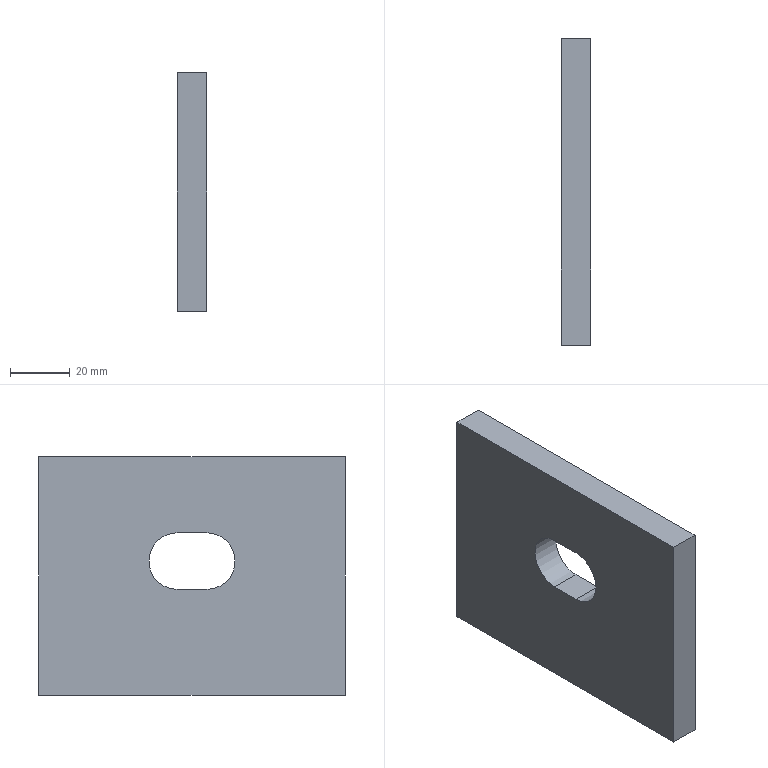Part | STEP file | VD-SYL0380DJ1006_1_5-4_VD-SYL03 | 1 solid | 10 faces | box 10 x 103 x 80 mm | volume 77665 mm3 | plane 8 | cylinder 2 | commonest cylinder face diameters 19 x2
STEP:
#1=CARTESIAN_POINT('',(0.,-46.5,-44.5));
#2=VERTEX_POINT('',#1);
#3=CARTESIAN_POINT('',(0.,-46.5,-25.5));
#4=VERTEX_POINT('',#3);
#5=CARTESIAN_POINT('',(0.,-46.5,-35.));
#6=DIRECTION('',(1.,0.,0.));
#7=DIRECTION('',(0.,0.,-1.));
#8=AXIS2_PLACEMENT_3D('',#5,#6,#7);
#9=CIRCLE('',#8,9.5);
#10=EDGE_CURVE('',#2,#4,#9,.T.);
#11=ORIENTED_EDGE('',*,*,#10,.T.);
#12=CARTESIAN_POINT('',(0.,-56.5,-25.5));
#13=VERTEX_POINT('',#12);
#14=CARTESIAN_POINT('',(0.,-46.5,-25.5));
#15=DIRECTION('',(0.,-1.,0.));
#16=VECTOR('',#15,1000.);
#17=LINE('',#14,#16);
#18=EDGE_CURVE('',#4,#13,#17,.T.);
#19=ORIENTED_EDGE('',*,*,#18,.T.);
#20=CARTESIAN_POINT('',(0.,-56.5,-44.5));
#21=VERTEX_POINT('',#20);
#22=CARTESIAN_POINT('',(0.,-56.5,-35.));
#23=DIRECTION('',(1.,0.,0.));
#24=DIRECTION('',(0.,0.,1.));
#25=AXIS2_PLACEMENT_3D('',#22,#23,#24);
#26=CIRCLE('',#25,9.5);
#27=EDGE_CURVE('',#13,#21,#26,.T.);
#28=ORIENTED_EDGE('',*,*,#27,.T.);
#29=CARTESIAN_POINT('',(0.,-56.5,-44.5));
#30=DIRECTION('',(0.,1.,0.));
#31=VECTOR('',#30,1000.);
#32=LINE('',#29,#31);
#33=EDGE_CURVE('',#21,#2,#32,.T.);
#34=ORIENTED_EDGE('',*,*,#33,.T.);
#35=EDGE_LOOP('',(#11,#19,#28,#34));
#36=FACE_BOUND('',#35,.T.);
#37=CARTESIAN_POINT('',(0.,-103.,-80.));
#38=VERTEX_POINT('',#37);
#39=CARTESIAN_POINT('',(0.,-103.,0.));
#40=VERTEX_POINT('',#39);
#41=CARTESIAN_POINT('',(0.,-103.,-80.));
#42=DIRECTION('',(0.,0.,1.));
#43=VECTOR('',#42,1000.);
#44=LINE('',#41,#43);
#45=EDGE_CURVE('',#38,#40,#44,.T.);
#46=ORIENTED_EDGE('',*,*,#45,.T.);
#47=CARTESIAN_POINT('',(0.,0.,0.));
#48=VERTEX_POINT('',#47);
#49=CARTESIAN_POINT('',(0.,-103.,0.));
#50=DIRECTION('',(0.,1.,0.));
#51=VECTOR('',#50,1000.);
#52=LINE('',#49,#51);
#53=EDGE_CURVE('',#40,#48,#52,.T.);
#54=ORIENTED_EDGE('',*,*,#53,.T.);
#55=CARTESIAN_POINT('',(0.,0.,-80.));
#56=VERTEX_POINT('',#55);
#57=CARTESIAN_POINT('',(0.,0.,0.));
#58=DIRECTION('',(0.,0.,-1.));
#59=VECTOR('',#58,1000.);
#60=LINE('',#57,#59);
#61=EDGE_CURVE('',#48,#56,#60,.T.);
#62=ORIENTED_EDGE('',*,*,#61,.T.);
#63=CARTESIAN_POINT('',(0.,0.,-80.));
#64=DIRECTION('',(0.,-1.,0.));
#65=VECTOR('',#64,1000.);
#66=LINE('',#63,#65);
#67=EDGE_CURVE('',#56,#38,#66,.T.);
#68=ORIENTED_EDGE('',*,*,#67,.T.);
#69=EDGE_LOOP('',(#46,#54,#62,#68));
#70=FACE_OUTER_BOUND('',#69,.T.);
#71=CARTESIAN_POINT('',(0.,0.,0.));
#72=DIRECTION('',(1.,0.,0.));
#73=DIRECTION('',(0.,1.,0.));
#74=AXIS2_PLACEMENT_3D('',#71,#72,#73);
#75=PLANE('',#74);
#76=ADVANCED_FACE('',(#36,#70),#75,.F.);
#77=CARTESIAN_POINT('',(10.,-46.5,-44.5));
#78=VERTEX_POINT('',#77);
#79=CARTESIAN_POINT('',(0.,-46.5,-44.5));
#80=DIRECTION('',(1.,0.,0.));
#81=VECTOR('',#80,1000.);
#82=LINE('',#79,#81);
#83=EDGE_CURVE('',#2,#78,#82,.T.);
#84=ORIENTED_EDGE('',*,*,#83,.F.);
#85=ORIENTED_EDGE('',*,*,#33,.F.);
#86=CARTESIAN_POINT('',(10.,-56.5,-44.5));
#87=VERTEX_POINT('',#86);
#88=CARTESIAN_POINT('',(10.,-56.5,-44.5));
#89=DIRECTION('',(-1.,0.,0.));
#90=VECTOR('',#89,1000.);
#91=LINE('',#88,#90);
#92=EDGE_CURVE('',#87,#21,#91,.T.);
#93=ORIENTED_EDGE('',*,*,#92,.F.);
#94=CARTESIAN_POINT('',(10.,-56.5,-44.5));
#95=DIRECTION('',(0.,1.,0.));
#96=VECTOR('',#95,1000.);
#97=LINE('',#94,#96);
#98=EDGE_CURVE('',#87,#78,#97,.T.);
#99=ORIENTED_EDGE('',*,*,#98,.T.);
#100=EDGE_LOOP('',(#84,#85,#93,#99));
#101=FACE_OUTER_BOUND('',#100,.T.);
#102=CARTESIAN_POINT('',(0.,-46.5,-44.5));
#103=DIRECTION('',(0.,0.,-1.));
#104=DIRECTION('',(0.,-1.,0.));
#105=AXIS2_PLACEMENT_3D('',#102,#103,#104);
#106=PLANE('',#105);
#107=ADVANCED_FACE('',(#101),#106,.F.);
#108=CARTESIAN_POINT('',(10.,-46.5,-25.5));
#109=VERTEX_POINT('',#108);
#110=CARTESIAN_POINT('',(10.,-46.5,-25.5));
#111=DIRECTION('',(-1.,0.,0.));
#112=VECTOR('',#111,1000.);
#113=LINE('',#110,#112);
#114=EDGE_CURVE('',#109,#4,#113,.T.);
#115=ORIENTED_EDGE('',*,*,#114,.T.);
#116=ORIENTED_EDGE('',*,*,#10,.F.);
#117=ORIENTED_EDGE('',*,*,#83,.T.);
#118=CARTESIAN_POINT('',(10.,-46.5,-35.));
#119=DIRECTION('',(-1.,0.,0.));
#120=DIRECTION('',(0.,0.,1.));
#121=AXIS2_PLACEMENT_3D('',#118,#119,#120);
#122=CIRCLE('',#121,9.5);
#123=EDGE_CURVE('',#109,#78,#122,.T.);
#124=ORIENTED_EDGE('',*,*,#123,.F.);
#125=EDGE_LOOP('',(#115,#116,#117,#124));
#126=FACE_OUTER_BOUND('',#125,.T.);
#127=CARTESIAN_POINT('',(0.,-46.5,-35.));
#128=DIRECTION('',(-1.,0.,0.));
#129=DIRECTION('',(0.,0.,1.));
#130=AXIS2_PLACEMENT_3D('',#127,#128,#129);
#131=CYLINDRICAL_SURFACE('',#130,9.5);
#132=ADVANCED_FACE('',(#126),#131,.F.);
#133=CARTESIAN_POINT('',(10.,-56.5,-25.5));
#134=VERTEX_POINT('',#133);
#135=CARTESIAN_POINT('',(0.,-56.5,-25.5));
#136=DIRECTION('',(1.,0.,0.));
#137=VECTOR('',#136,1000.);
#138=LINE('',#135,#137);
#139=EDGE_CURVE('',#13,#134,#138,.T.);
#140=ORIENTED_EDGE('',*,*,#139,.F.);
#141=ORIENTED_EDGE('',*,*,#18,.F.);
#142=ORIENTED_EDGE('',*,*,#114,.F.);
#143=CARTESIAN_POINT('',(10.,-46.5,-25.5));
#144=DIRECTION('',(0.,-1.,0.));
#145=VECTOR('',#144,1000.);
#146=LINE('',#143,#145);
#147=EDGE_CURVE('',#109,#134,#146,.T.);
#148=ORIENTED_EDGE('',*,*,#147,.T.);
#149=EDGE_LOOP('',(#140,#141,#142,#148));
#150=FACE_OUTER_BOUND('',#149,.T.);
#151=CARTESIAN_POINT('',(0.,-56.5,-25.5));
#152=DIRECTION('',(0.,0.,1.));
#153=DIRECTION('',(1.,0.,0.));
#154=AXIS2_PLACEMENT_3D('',#151,#152,#153);
#155=PLANE('',#154);
#156=ADVANCED_FACE('',(#150),#155,.F.);
#157=ORIENTED_EDGE('',*,*,#92,.T.);
#158=ORIENTED_EDGE('',*,*,#27,.F.);
#159=ORIENTED_EDGE('',*,*,#139,.T.);
#160=CARTESIAN_POINT('',(10.,-56.5,-35.));
#161=DIRECTION('',(-1.,0.,0.));
#162=DIRECTION('',(0.,0.,-1.));
#163=AXIS2_PLACEMENT_3D('',#160,#161,#162);
#164=CIRCLE('',#163,9.5);
#165=EDGE_CURVE('',#87,#134,#164,.T.);
#166=ORIENTED_EDGE('',*,*,#165,.F.);
#167=EDGE_LOOP('',(#157,#158,#159,#166));
#168=FACE_OUTER_BOUND('',#167,.T.);
#169=CARTESIAN_POINT('',(0.,-56.5,-35.));
#170=DIRECTION('',(-1.,0.,0.));
#171=DIRECTION('',(0.,0.,1.));
#172=AXIS2_PLACEMENT_3D('',#169,#170,#171);
#173=CYLINDRICAL_SURFACE('',#172,9.5);
#174=ADVANCED_FACE('',(#168),#173,.F.);
#175=ORIENTED_EDGE('',*,*,#147,.F.);
#176=ORIENTED_EDGE('',*,*,#123,.T.);
#177=ORIENTED_EDGE('',*,*,#98,.F.);
#178=ORIENTED_EDGE('',*,*,#165,.T.);
#179=EDGE_LOOP('',(#175,#176,#177,#178));
#180=FACE_BOUND('',#179,.T.);
#181=CARTESIAN_POINT('',(10.,0.,0.));
#182=VERTEX_POINT('',#181);
#183=CARTESIAN_POINT('',(10.,-103.,0.));
#184=VERTEX_POINT('',#183);
#185=CARTESIAN_POINT('',(10.,0.,0.));
#186=DIRECTION('',(0.,-1.,0.));
#187=VECTOR('',#186,1000.);
#188=LINE('',#185,#187);
#189=EDGE_CURVE('',#182,#184,#188,.T.);
#190=ORIENTED_EDGE('',*,*,#189,.T.);
#191=CARTESIAN_POINT('',(10.,-103.,-80.));
#192=VERTEX_POINT('',#191);
#193=CARTESIAN_POINT('',(10.,-103.,0.));
#194=DIRECTION('',(0.,0.,-1.));
#195=VECTOR('',#194,1000.);
#196=LINE('',#193,#195);
#197=EDGE_CURVE('',#184,#192,#196,.T.);
#198=ORIENTED_EDGE('',*,*,#197,.T.);
#199=CARTESIAN_POINT('',(10.,0.,-80.));
#200=VERTEX_POINT('',#199);
#201=CARTESIAN_POINT('',(10.,-103.,-80.));
#202=DIRECTION('',(0.,1.,0.));
#203=VECTOR('',#202,1000.);
#204=LINE('',#201,#203);
#205=EDGE_CURVE('',#192,#200,#204,.T.);
#206=ORIENTED_EDGE('',*,*,#205,.T.);
#207=CARTESIAN_POINT('',(10.,0.,-80.));
#208=DIRECTION('',(0.,0.,1.));
#209=VECTOR('',#208,1000.);
#210=LINE('',#207,#209);
#211=EDGE_CURVE('',#200,#182,#210,.T.);
#212=ORIENTED_EDGE('',*,*,#211,.T.);
#213=EDGE_LOOP('',(#190,#198,#206,#212));
#214=FACE_OUTER_BOUND('',#213,.T.);
#215=CARTESIAN_POINT('',(10.,0.,0.));
#216=DIRECTION('',(1.,0.,0.));
#217=DIRECTION('',(0.,1.,0.));
#218=AXIS2_PLACEMENT_3D('',#215,#216,#217);
#219=PLANE('',#218);
#220=ADVANCED_FACE('',(#180,#214),#219,.T.);
#221=ORIENTED_EDGE('',*,*,#45,.F.);
#222=CARTESIAN_POINT('',(0.,-103.,-80.));
#223=DIRECTION('',(1.,0.,0.));
#224=VECTOR('',#223,1000.);
#225=LINE('',#222,#224);
#226=EDGE_CURVE('',#38,#192,#225,.T.);
#227=ORIENTED_EDGE('',*,*,#226,.T.);
#228=ORIENTED_EDGE('',*,*,#197,.F.);
#229=CARTESIAN_POINT('',(0.,-103.,0.));
#230=DIRECTION('',(1.,0.,0.));
#231=VECTOR('',#230,1000.);
#232=LINE('',#229,#231);
#233=EDGE_CURVE('',#40,#184,#232,.T.);
#234=ORIENTED_EDGE('',*,*,#233,.F.);
#235=EDGE_LOOP('',(#221,#227,#228,#234));
#236=FACE_OUTER_BOUND('',#235,.T.);
#237=CARTESIAN_POINT('',(0.,-103.,0.));
#238=DIRECTION('',(0.,-1.,0.));
#239=DIRECTION('',(0.,0.,-1.));
#240=AXIS2_PLACEMENT_3D('',#237,#238,#239);
#241=PLANE('',#240);
#242=ADVANCED_FACE('',(#236),#241,.T.);
#243=ORIENTED_EDGE('',*,*,#67,.F.);
#244=CARTESIAN_POINT('',(0.,0.,-80.));
#245=DIRECTION('',(1.,0.,0.));
#246=VECTOR('',#245,1000.);
#247=LINE('',#244,#246);
#248=EDGE_CURVE('',#56,#200,#247,.T.);
#249=ORIENTED_EDGE('',*,*,#248,.T.);
#250=ORIENTED_EDGE('',*,*,#205,.F.);
#251=ORIENTED_EDGE('',*,*,#226,.F.);
#252=EDGE_LOOP('',(#243,#249,#250,#251));
#253=FACE_OUTER_BOUND('',#252,.T.);
#254=CARTESIAN_POINT('',(0.,-103.,-80.));
#255=DIRECTION('',(0.,0.,-1.));
#256=DIRECTION('',(0.,-1.,0.));
#257=AXIS2_PLACEMENT_3D('',#254,#255,#256);
#258=PLANE('',#257);
#259=ADVANCED_FACE('',(#253),#258,.T.);
#260=ORIENTED_EDGE('',*,*,#61,.F.);
#261=CARTESIAN_POINT('',(10.,0.,0.));
#262=DIRECTION('',(-1.,0.,0.));
#263=VECTOR('',#262,1000.);
#264=LINE('',#261,#263);
#265=EDGE_CURVE('',#182,#48,#264,.T.);
#266=ORIENTED_EDGE('',*,*,#265,.F.);
#267=ORIENTED_EDGE('',*,*,#211,.F.);
#268=ORIENTED_EDGE('',*,*,#248,.F.);
#269=EDGE_LOOP('',(#260,#266,#267,#268));
#270=FACE_OUTER_BOUND('',#269,.T.);
#271=CARTESIAN_POINT('',(0.,0.,-80.));
#272=DIRECTION('',(0.,1.,0.));
#273=DIRECTION('',(1.,0.,0.));
#274=AXIS2_PLACEMENT_3D('',#271,#272,#273);
#275=PLANE('',#274);
#276=ADVANCED_FACE('',(#270),#275,.T.);
#277=ORIENTED_EDGE('',*,*,#53,.F.);
#278=ORIENTED_EDGE('',*,*,#233,.T.);
#279=ORIENTED_EDGE('',*,*,#189,.F.);
#280=ORIENTED_EDGE('',*,*,#265,.T.);
#281=EDGE_LOOP('',(#277,#278,#279,#280));
#282=FACE_OUTER_BOUND('',#281,.T.);
#283=CARTESIAN_POINT('',(0.,0.,0.));
#284=DIRECTION('',(0.,0.,1.));
#285=DIRECTION('',(1.,0.,0.));
#286=AXIS2_PLACEMENT_3D('',#283,#284,#285);
#287=PLANE('',#286);
#288=ADVANCED_FACE('',(#282),#287,.T.);
#289=CLOSED_SHELL('',(#76,#107,#132,#156,#174,#220,#242,#259,#276,#288));
#290=MANIFOLD_SOLID_BREP('',#289);
#291=CARTESIAN_POINT('',(0.,0.,0.));
#292=DIRECTION('',(0.,0.,1.));
#293=DIRECTION('',(1.,0.,0.));
#294=AXIS2_PLACEMENT_3D('',#291,#292,#293);
#295=(LENGTH_UNIT()NAMED_UNIT(*)SI_UNIT(.MILLI.,.METRE.));
#296=UNCERTAINTY_MEASURE_WITH_UNIT(LENGTH_MEASURE(0.00001),#295,'','');
#297=(NAMED_UNIT(*)PLANE_ANGLE_UNIT()SI_UNIT($,.RADIAN.));
#298=(NAMED_UNIT(*)SI_UNIT($,.STERADIAN.)SOLID_ANGLE_UNIT());
#299=(GEOMETRIC_REPRESENTATION_CONTEXT(3)GLOBAL_UNCERTAINTY_ASSIGNED_CONTEXT((#296))GLOBAL_UNIT_ASSIGNED_CONTEXT((#295,#297,#298))REPRESENTATION_CONTEXT('',''));
#300=ADVANCED_BREP_SHAPE_REPRESENTATION('',(#290,#294),#299);